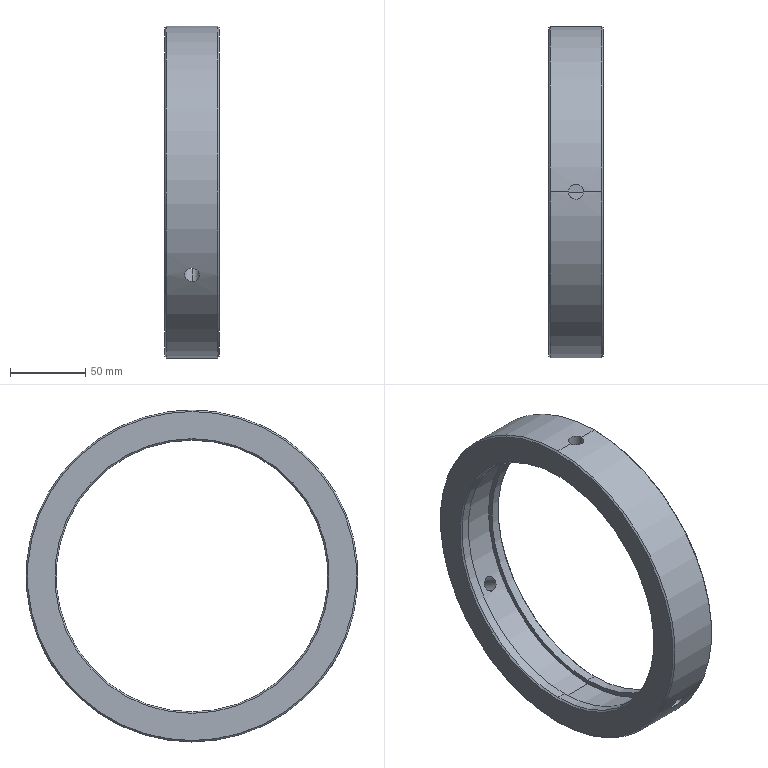Part | SolidWorks | features 3DProfileFeature 1, Chamfer 1, CirPattern 1, HoleWzd 1, Revolution 1 | 1 solid | 26 faces | box 36 x 220 x 220 mm | volume 409173 mm3 | cylinder 14 | cone 8 | plane 4 | commonest cylinder face diameters 10 x6 180 x4 186 x2 220 x2
STEP:
#1=CARTESIAN_POINT('',(0.,-82.924,-42.103));
#2=VERTEX_POINT('',#1);
#3=CARTESIAN_POINT('',(0.,-77.924,-50.763));
#4=VERTEX_POINT('',#3);
#5=CARTESIAN_POINT('',(0.,-82.924,-42.103));
#6=CARTESIAN_POINT('',(-0.3263,-82.924,-42.103));
#7=CARTESIAN_POINT('',(-0.6506,-82.91,-42.131));
#8=CARTESIAN_POINT('',(-1.295,-82.851,-42.245));
#9=CARTESIAN_POINT('',(-1.611,-82.808,-42.331));
#10=CARTESIAN_POINT('',(-2.213,-82.694,-42.553));
#11=CARTESIAN_POINT('',(-2.503,-82.623,-42.69));
#12=CARTESIAN_POINT('',(-3.051,-82.455,-43.015));
#13=CARTESIAN_POINT('',(-3.302,-82.359,-43.198));
#14=CARTESIAN_POINT('',(-3.764,-82.144,-43.606));
#15=CARTESIAN_POINT('',(-3.975,-82.023,-43.833));
#16=CARTESIAN_POINT('',(-4.338,-81.765,-44.312));
#17=CARTESIAN_POINT('',(-4.492,-81.628,-44.564));
#18=CARTESIAN_POINT('',(-4.743,-81.336,-45.094));
#19=CARTESIAN_POINT('',(-4.84,-81.182,-45.372));
#20=CARTESIAN_POINT('',(-4.967,-80.868,-45.929));
#21=CARTESIAN_POINT('',(-5.,-80.707,-46.211));
#22=CARTESIAN_POINT('',(-5.,-80.378,-46.782));
#23=CARTESIAN_POINT('',(-4.968,-80.213,-47.064));
#24=CARTESIAN_POINT('',(-4.873,-79.969,-47.476));
#25=CARTESIAN_POINT('',(-4.834,-79.888,-47.612));
#26=CARTESIAN_POINT('',(-4.739,-79.727,-47.882));
#27=CARTESIAN_POINT('',(-4.683,-79.646,-48.015));
#28=CARTESIAN_POINT('',(-4.495,-79.411,-48.405));
#29=CARTESIAN_POINT('',(-4.342,-79.261,-48.65));
#30=CARTESIAN_POINT('',(-3.98,-78.975,-49.112));
#31=CARTESIAN_POINT('',(-3.769,-78.839,-49.331));
#32=CARTESIAN_POINT('',(-3.307,-78.593,-49.722));
#33=CARTESIAN_POINT('',(-3.056,-78.482,-49.897));
#34=CARTESIAN_POINT('',(-2.511,-78.285,-50.205));
#35=CARTESIAN_POINT('',(-2.219,-78.2,-50.336));
#36=CARTESIAN_POINT('',(-1.618,-78.065,-50.546));
#37=CARTESIAN_POINT('',(-1.304,-78.012,-50.627));
#38=CARTESIAN_POINT('',(-0.6572,-77.942,-50.736));
#39=CARTESIAN_POINT('',(-0.3304,-77.924,-50.763));
#40=CARTESIAN_POINT('',(0.,-77.924,-50.763));
#41=B_SPLINE_CURVE_WITH_KNOTS('',3,(#5,#6,#7,#8,#9,#10,#11,#12,#13,#14,#15,#16,#17,#18,#19,#20,#21,#22,#23,#24,#25,#26,#27,#28,#29,#30,#31,#32,#33,#34,#35,#36,#37,#38,#39,#40),.UNSPECIFIED.,.F.,.F.,(4,2,2,2,2,2,2,2,2,2,2,2,2,2,2,2,2,4),(0.01564,0.01661,0.01759,0.01857,0.01954,0.02052,0.0215,0.02247,0.02345,0.02443,0.02492,0.0254,0.02638,0.02736,0.02834,0.02931,0.03029,0.03127),.UNSPECIFIED.);
#42=EDGE_CURVE('',#2,#4,#41,.T.);
#43=ORIENTED_EDGE('',*,*,#42,.F.);
#44=CARTESIAN_POINT('',(0.,-97.664,-50.613));
#45=VERTEX_POINT('',#44);
#46=CARTESIAN_POINT('',(0.,-97.763,-50.67));
#47=DIRECTION('',(0.,-0.866,-0.5));
#48=VECTOR('',#47,1000.);
#49=LINE('',#46,#48);
#50=EDGE_CURVE('',#2,#45,#49,.T.);
#51=ORIENTED_EDGE('',*,*,#50,.T.);
#52=CARTESIAN_POINT('',(0.,-92.664,-59.273));
#53=VERTEX_POINT('',#52);
#54=CARTESIAN_POINT('',(0.,-92.664,-59.273));
#55=CARTESIAN_POINT('',(-0.3304,-92.664,-59.273));
#56=CARTESIAN_POINT('',(-0.6553,-92.682,-59.246));
#57=CARTESIAN_POINT('',(-1.135,-92.733,-59.166));
#58=CARTESIAN_POINT('',(-1.293,-92.754,-59.132));
#59=CARTESIAN_POINT('',(-1.607,-92.806,-59.052));
#60=CARTESIAN_POINT('',(-1.763,-92.836,-59.005));
#61=CARTESIAN_POINT('',(-2.218,-92.937,-58.845));
#62=CARTESIAN_POINT('',(-2.505,-93.019,-58.716));
#63=CARTESIAN_POINT('',(-3.048,-93.212,-58.408));
#64=CARTESIAN_POINT('',(-3.306,-93.324,-58.229));
#65=CARTESIAN_POINT('',(-3.767,-93.568,-57.837));
#66=CARTESIAN_POINT('',(-3.974,-93.7,-57.623));
#67=CARTESIAN_POINT('',(-4.339,-93.985,-57.156));
#68=CARTESIAN_POINT('',(-4.495,-94.136,-56.907));
#69=CARTESIAN_POINT('',(-4.744,-94.446,-56.391));
#70=CARTESIAN_POINT('',(-4.84,-94.608,-56.12));
#71=CARTESIAN_POINT('',(-4.968,-94.935,-55.564));
#72=CARTESIAN_POINT('',(-5.,-95.099,-55.284));
#73=CARTESIAN_POINT('',(-5.,-95.425,-54.719));
#74=CARTESIAN_POINT('',(-4.968,-95.589,-54.431));
#75=CARTESIAN_POINT('',(-4.84,-95.905,-53.873));
#76=CARTESIAN_POINT('',(-4.745,-96.057,-53.601));
#77=CARTESIAN_POINT('',(-4.495,-96.351,-53.072));
#78=CARTESIAN_POINT('',(-4.338,-96.492,-52.815));
#79=CARTESIAN_POINT('',(-3.976,-96.751,-52.339));
#80=CARTESIAN_POINT('',(-3.77,-96.871,-52.116));
#81=CARTESIAN_POINT('',(-3.303,-97.091,-51.705));
#82=CARTESIAN_POINT('',(-3.05,-97.188,-51.521));
#83=CARTESIAN_POINT('',(-2.644,-97.315,-51.281));
#84=CARTESIAN_POINT('',(-2.504,-97.354,-51.207));
#85=CARTESIAN_POINT('',(-2.215,-97.426,-51.069));
#86=CARTESIAN_POINT('',(-2.065,-97.459,-51.007));
#87=CARTESIAN_POINT('',(-1.61,-97.547,-50.84));
#88=CARTESIAN_POINT('',(-1.299,-97.59,-50.756));
#89=CARTESIAN_POINT('',(-0.6578,-97.649,-50.642));
#90=CARTESIAN_POINT('',(-0.3263,-97.664,-50.613));
#91=CARTESIAN_POINT('',(0.,-97.664,-50.613));
#92=B_SPLINE_CURVE_WITH_KNOTS('',3,(#54,#55,#56,#57,#58,#59,#60,#61,#62,#63,#64,#65,#66,#67,#68,#69,#70,#71,#72,#73,#74,#75,#76,#77,#78,#79,#80,#81,#82,#83,#84,#85,#86,#87,#88,#89,#90,#91),.UNSPECIFIED.,.F.,.F.,(4,2,2,2,2,2,2,2,2,2,2,2,2,2,2,2,2,2,4),(0.,0.0009771,0.001466,0.001954,0.002931,0.003909,0.004886,0.005863,0.00684,0.007817,0.008794,0.009771,0.01075,0.01173,0.0127,0.01319,0.01368,0.01466,0.01563),.UNSPECIFIED.);
#93=EDGE_CURVE('',#53,#45,#92,.T.);
#94=ORIENTED_EDGE('',*,*,#93,.F.);
#95=CARTESIAN_POINT('',(0.,-92.763,-59.33));
#96=DIRECTION('',(0.,-0.866,-0.5));
#97=VECTOR('',#96,1000.);
#98=LINE('',#95,#97);
#99=EDGE_CURVE('',#4,#53,#98,.T.);
#100=ORIENTED_EDGE('',*,*,#99,.F.);
#101=EDGE_LOOP('',(#43,#51,#94,#100));
#102=FACE_OUTER_BOUND('',#101,.T.);
#103=CARTESIAN_POINT('',(0.,-95.263,-55.));
#104=DIRECTION('',(0.,-0.866,-0.5));
#105=DIRECTION('',(0.,0.5,-0.866));
#106=AXIS2_PLACEMENT_3D('',#103,#104,#105);
#107=CYLINDRICAL_SURFACE('',#106,5.);
#108=ADVANCED_FACE('',(#102),#107,.F.);
#109=CARTESIAN_POINT('',(0.,77.924,-50.763));
#110=VERTEX_POINT('',#109);
#111=CARTESIAN_POINT('',(0.,82.924,-42.103));
#112=VERTEX_POINT('',#111);
#113=CARTESIAN_POINT('',(0.,77.924,-50.763));
#114=CARTESIAN_POINT('',(-0.3263,77.924,-50.763));
#115=CARTESIAN_POINT('',(-0.6506,77.941,-50.736));
#116=CARTESIAN_POINT('',(-1.295,78.011,-50.629));
#117=CARTESIAN_POINT('',(-1.611,78.063,-50.548));
#118=CARTESIAN_POINT('',(-2.213,78.199,-50.339));
#119=CARTESIAN_POINT('',(-2.503,78.282,-50.209));
#120=CARTESIAN_POINT('',(-3.051,78.479,-49.9));
#121=CARTESIAN_POINT('',(-3.302,78.59,-49.725));
#122=CARTESIAN_POINT('',(-3.764,78.836,-49.335));
#123=CARTESIAN_POINT('',(-3.975,78.972,-49.117));
#124=CARTESIAN_POINT('',(-4.338,79.258,-48.655));
#125=CARTESIAN_POINT('',(-4.492,79.408,-48.41));
#126=CARTESIAN_POINT('',(-4.743,79.721,-47.892));
#127=CARTESIAN_POINT('',(-4.84,79.884,-47.62));
#128=CARTESIAN_POINT('',(-4.967,80.21,-47.069));
#129=CARTESIAN_POINT('',(-5.,80.373,-46.789));
#130=CARTESIAN_POINT('',(-5.,80.703,-46.218));
#131=CARTESIAN_POINT('',(-4.968,80.865,-45.935));
#132=CARTESIAN_POINT('',(-4.873,81.1,-45.517));
#133=CARTESIAN_POINT('',(-4.834,81.177,-45.379));
#134=CARTESIAN_POINT('',(-4.739,81.33,-45.105));
#135=CARTESIAN_POINT('',(-4.683,81.406,-44.968));
#136=CARTESIAN_POINT('',(-4.495,81.625,-44.57));
#137=CARTESIAN_POINT('',(-4.342,81.762,-44.317));
#138=CARTESIAN_POINT('',(-3.98,82.02,-43.839));
#139=CARTESIAN_POINT('',(-3.769,82.141,-43.611));
#140=CARTESIAN_POINT('',(-3.307,82.357,-43.202));
#141=CARTESIAN_POINT('',(-3.056,82.453,-43.019));
#142=CARTESIAN_POINT('',(-2.511,82.621,-42.694));
#143=CARTESIAN_POINT('',(-2.219,82.693,-42.555));
#144=CARTESIAN_POINT('',(-1.618,82.807,-42.333));
#145=CARTESIAN_POINT('',(-1.304,82.85,-42.247));
#146=CARTESIAN_POINT('',(-0.6572,82.909,-42.132));
#147=CARTESIAN_POINT('',(-0.3304,82.924,-42.103));
#148=CARTESIAN_POINT('',(0.,82.924,-42.103));
#149=B_SPLINE_CURVE_WITH_KNOTS('',3,(#113,#114,#115,#116,#117,#118,#119,#120,#121,#122,#123,#124,#125,#126,#127,#128,#129,#130,#131,#132,#133,#134,#135,#136,#137,#138,#139,#140,#141,#142,#143,#144,#145,#146,#147,#148),.UNSPECIFIED.,.F.,.F.,(4,2,2,2,2,2,2,2,2,2,2,2,2,2,2,2,2,4),(0.01564,0.01661,0.01759,0.01857,0.01954,0.02052,0.0215,0.02247,0.02345,0.02443,0.02492,0.0254,0.02638,0.02736,0.02834,0.02931,0.03029,0.03127),.UNSPECIFIED.);
#150=EDGE_CURVE('',#110,#112,#149,.T.);
#151=ORIENTED_EDGE('',*,*,#150,.F.);
#152=CARTESIAN_POINT('',(0.,92.664,-59.273));
#153=VERTEX_POINT('',#152);
#154=CARTESIAN_POINT('',(0.,92.763,-59.33));
#155=DIRECTION('',(0.,0.866,-0.5));
#156=VECTOR('',#155,1000.);
#157=LINE('',#154,#156);
#158=EDGE_CURVE('',#110,#153,#157,.T.);
#159=ORIENTED_EDGE('',*,*,#158,.T.);
#160=CARTESIAN_POINT('',(0.,97.664,-50.613));
#161=VERTEX_POINT('',#160);
#162=CARTESIAN_POINT('',(0.,97.664,-50.613));
#163=CARTESIAN_POINT('',(-0.3304,97.664,-50.613));
#164=CARTESIAN_POINT('',(-0.6553,97.649,-50.642));
#165=CARTESIAN_POINT('',(-1.135,97.605,-50.727));
#166=CARTESIAN_POINT('',(-1.293,97.587,-50.762));
#167=CARTESIAN_POINT('',(-1.607,97.543,-50.846));
#168=CARTESIAN_POINT('',(-1.763,97.517,-50.896));
#169=CARTESIAN_POINT('',(-2.218,97.43,-51.063));
#170=CARTESIAN_POINT('',(-2.505,97.359,-51.199));
#171=CARTESIAN_POINT('',(-3.048,97.189,-51.52));
#172=CARTESIAN_POINT('',(-3.306,97.09,-51.707));
#173=CARTESIAN_POINT('',(-3.767,96.872,-52.114));
#174=CARTESIAN_POINT('',(-3.974,96.753,-52.335));
#175=CARTESIAN_POINT('',(-4.339,96.491,-52.816));
#176=CARTESIAN_POINT('',(-4.495,96.351,-53.071));
#177=CARTESIAN_POINT('',(-4.744,96.059,-53.597));
#178=CARTESIAN_POINT('',(-4.84,95.906,-53.872));
#179=CARTESIAN_POINT('',(-4.968,95.588,-54.434));
#180=CARTESIAN_POINT('',(-5.,95.427,-54.716));
#181=CARTESIAN_POINT('',(-5.,95.101,-55.281));
#182=CARTESIAN_POINT('',(-4.968,94.934,-55.567));
#183=CARTESIAN_POINT('',(-4.84,94.608,-56.12));
#184=CARTESIAN_POINT('',(-4.745,94.449,-56.388));
#185=CARTESIAN_POINT('',(-4.495,94.137,-56.907));
#186=CARTESIAN_POINT('',(-4.338,93.985,-57.157));
#187=CARTESIAN_POINT('',(-3.976,93.702,-57.619));
#188=CARTESIAN_POINT('',(-3.77,93.569,-57.834));
#189=CARTESIAN_POINT('',(-3.303,93.323,-58.231));
#190=CARTESIAN_POINT('',(-3.05,93.213,-58.407));
#191=CARTESIAN_POINT('',(-2.644,93.068,-58.637));
#192=CARTESIAN_POINT('',(-2.504,93.023,-58.708));
#193=CARTESIAN_POINT('',(-2.215,92.941,-58.839));
#194=CARTESIAN_POINT('',(-2.065,92.903,-58.899));
#195=CARTESIAN_POINT('',(-1.61,92.802,-59.058));
#196=CARTESIAN_POINT('',(-1.299,92.751,-59.138));
#197=CARTESIAN_POINT('',(-0.6578,92.682,-59.246));
#198=CARTESIAN_POINT('',(-0.3263,92.664,-59.273));
#199=CARTESIAN_POINT('',(0.,92.664,-59.273));
#200=B_SPLINE_CURVE_WITH_KNOTS('',3,(#162,#163,#164,#165,#166,#167,#168,#169,#170,#171,#172,#173,#174,#175,#176,#177,#178,#179,#180,#181,#182,#183,#184,#185,#186,#187,#188,#189,#190,#191,#192,#193,#194,#195,#196,#197,#198,#199),.UNSPECIFIED.,.F.,.F.,(4,2,2,2,2,2,2,2,2,2,2,2,2,2,2,2,2,2,4),(0.,0.0009771,0.001466,0.001954,0.002931,0.003909,0.004886,0.005863,0.00684,0.007817,0.008794,0.009771,0.01075,0.01173,0.0127,0.01319,0.01368,0.01466,0.01563),.UNSPECIFIED.);
#201=EDGE_CURVE('',#161,#153,#200,.T.);
#202=ORIENTED_EDGE('',*,*,#201,.F.);
#203=CARTESIAN_POINT('',(0.,97.763,-50.67));
#204=DIRECTION('',(0.,0.866,-0.5));
#205=VECTOR('',#204,1000.);
#206=LINE('',#203,#205);
#207=EDGE_CURVE('',#112,#161,#206,.T.);
#208=ORIENTED_EDGE('',*,*,#207,.F.);
#209=EDGE_LOOP('',(#151,#159,#202,#208));
#210=FACE_OUTER_BOUND('',#209,.T.);
#211=CARTESIAN_POINT('',(0.,95.263,-55.));
#212=DIRECTION('',(0.,0.866,-0.5));
#213=DIRECTION('',(0.,0.5,0.866));
#214=AXIS2_PLACEMENT_3D('',#211,#212,#213);
#215=CYLINDRICAL_SURFACE('',#214,5.);
#216=ADVANCED_FACE('',(#210),#215,.F.);
#217=CARTESIAN_POINT('',(-5.,0.,93.));
#218=VERTEX_POINT('',#217);
#219=CARTESIAN_POINT('',(5.,0.,93.));
#220=VERTEX_POINT('',#219);
#221=CARTESIAN_POINT('',(-5.,0.,93.));
#222=CARTESIAN_POINT('',(-5.,-0.3263,93.));
#223=CARTESIAN_POINT('',(-4.968,-0.6506,92.998));
#224=CARTESIAN_POINT('',(-4.84,-1.295,92.992));
#225=CARTESIAN_POINT('',(-4.744,-1.611,92.987));
#226=CARTESIAN_POINT('',(-4.495,-2.213,92.974));
#227=CARTESIAN_POINT('',(-4.341,-2.503,92.967));
#228=CARTESIAN_POINT('',(-3.975,-3.051,92.95));
#229=CARTESIAN_POINT('',(-3.768,-3.302,92.942));
#230=CARTESIAN_POINT('',(-3.308,-3.764,92.924));
#231=CARTESIAN_POINT('',(-3.051,-3.975,92.915));
#232=CARTESIAN_POINT('',(-2.507,-4.338,92.899));
#233=CARTESIAN_POINT('',(-2.22,-4.492,92.892));
#234=CARTESIAN_POINT('',(-1.616,-4.743,92.879));
#235=CARTESIAN_POINT('',(-1.298,-4.84,92.874));
#236=CARTESIAN_POINT('',(-0.6586,-4.967,92.867));
#237=CARTESIAN_POINT('',(-0.3339,-5.,92.866));
#238=CARTESIAN_POINT('',(0.3257,-5.,92.865));
#239=CARTESIAN_POINT('',(0.6518,-4.968,92.867));
#240=CARTESIAN_POINT('',(1.131,-4.873,92.872));
#241=CARTESIAN_POINT('',(1.289,-4.834,92.874));
#242=CARTESIAN_POINT('',(1.603,-4.739,92.879));
#243=CARTESIAN_POINT('',(1.759,-4.683,92.882));
#244=CARTESIAN_POINT('',(2.214,-4.495,92.891));
#245=CARTESIAN_POINT('',(2.501,-4.342,92.899));
#246=CARTESIAN_POINT('',(3.045,-3.98,92.915));
#247=CARTESIAN_POINT('',(3.302,-3.769,92.924));
#248=CARTESIAN_POINT('',(3.764,-3.307,92.941));
#249=CARTESIAN_POINT('',(3.971,-3.056,92.95));
#250=CARTESIAN_POINT('',(4.336,-2.511,92.967));
#251=CARTESIAN_POINT('',(4.492,-2.219,92.974));
#252=CARTESIAN_POINT('',(4.742,-1.618,92.986));
#253=CARTESIAN_POINT('',(4.838,-1.304,92.991));
#254=CARTESIAN_POINT('',(4.968,-0.6572,92.998));
#255=CARTESIAN_POINT('',(5.,-0.3304,93.));
#256=CARTESIAN_POINT('',(5.,0.,93.));
#257=B_SPLINE_CURVE_WITH_KNOTS('',3,(#221,#222,#223,#224,#225,#226,#227,#228,#229,#230,#231,#232,#233,#234,#235,#236,#237,#238,#239,#240,#241,#242,#243,#244,#245,#246,#247,#248,#249,#250,#251,#252,#253,#254,#255,#256),.UNSPECIFIED.,.F.,.F.,(4,2,2,2,2,2,2,2,2,2,2,2,2,2,2,2,2,4),(0.01564,0.01661,0.01759,0.01857,0.01954,0.02052,0.0215,0.02247,0.02345,0.02443,0.02492,0.0254,0.02638,0.02736,0.02834,0.02931,0.03029,0.03127),.UNSPECIFIED.);
#258=EDGE_CURVE('',#218,#220,#257,.T.);
#259=ORIENTED_EDGE('',*,*,#258,.F.);
#260=CARTESIAN_POINT('',(-5.,0.,110.));
#261=VERTEX_POINT('',#260);
#262=CARTESIAN_POINT('',(-5.,0.,110.));
#263=DIRECTION('',(0.,0.,1.));
#264=VECTOR('',#263,1000.);
#265=LINE('',#262,#264);
#266=EDGE_CURVE('',#218,#261,#265,.T.);
#267=ORIENTED_EDGE('',*,*,#266,.T.);
#268=CARTESIAN_POINT('',(5.,0.,110.));
#269=VERTEX_POINT('',#268);
#270=CARTESIAN_POINT('',(5.,0.,110.));
#271=CARTESIAN_POINT('',(5.,-0.3304,110.));
#272=CARTESIAN_POINT('',(4.968,-0.6553,109.999));
#273=CARTESIAN_POINT('',(4.872,-1.135,109.994));
#274=CARTESIAN_POINT('',(4.833,-1.293,109.993));
#275=CARTESIAN_POINT('',(4.737,-1.607,109.988));
#276=CARTESIAN_POINT('',(4.682,-1.763,109.986));
#277=CARTESIAN_POINT('',(4.493,-2.218,109.978));
#278=CARTESIAN_POINT('',(4.34,-2.505,109.972));
#279=CARTESIAN_POINT('',(3.977,-3.048,109.958));
#280=CARTESIAN_POINT('',(3.766,-3.306,109.951));
#281=CARTESIAN_POINT('',(3.304,-3.767,109.936));
#282=CARTESIAN_POINT('',(3.052,-3.974,109.928));
#283=CARTESIAN_POINT('',(2.506,-4.339,109.915));
#284=CARTESIAN_POINT('',(2.215,-4.495,109.908));
#285=CARTESIAN_POINT('',(1.613,-4.744,109.898));
#286=CARTESIAN_POINT('',(1.298,-4.84,109.893));
#287=CARTESIAN_POINT('',(0.6524,-4.968,109.888));
#288=CARTESIAN_POINT('',(0.3279,-5.,109.886));
#289=CARTESIAN_POINT('',(-0.3244,-5.,109.886));
#290=CARTESIAN_POINT('',(-0.6557,-4.968,109.888));
#291=CARTESIAN_POINT('',(-1.297,-4.84,109.893));
#292=CARTESIAN_POINT('',(-1.609,-4.745,109.898));
#293=CARTESIAN_POINT('',(-2.214,-4.495,109.908));
#294=CARTESIAN_POINT('',(-2.507,-4.338,109.915));
#295=CARTESIAN_POINT('',(-3.049,-3.976,109.928));
#296=CARTESIAN_POINT('',(-3.301,-3.77,109.936));
#297=CARTESIAN_POINT('',(-3.768,-3.303,109.951));
#298=CARTESIAN_POINT('',(-3.975,-3.05,109.958));
#299=CARTESIAN_POINT('',(-4.247,-2.644,109.968));
#300=CARTESIAN_POINT('',(-4.331,-2.504,109.972));
#301=CARTESIAN_POINT('',(-4.486,-2.215,109.978));
#302=CARTESIAN_POINT('',(-4.557,-2.065,109.981));
#303=CARTESIAN_POINT('',(-4.745,-1.61,109.989));
#304=CARTESIAN_POINT('',(-4.839,-1.299,109.993));
#305=CARTESIAN_POINT('',(-4.967,-0.6578,109.998));
#306=CARTESIAN_POINT('',(-5.,-0.3263,110.));
#307=CARTESIAN_POINT('',(-5.,0.,110.));
#308=B_SPLINE_CURVE_WITH_KNOTS('',3,(#270,#271,#272,#273,#274,#275,#276,#277,#278,#279,#280,#281,#282,#283,#284,#285,#286,#287,#288,#289,#290,#291,#292,#293,#294,#295,#296,#297,#298,#299,#300,#301,#302,#303,#304,#305,#306,#307),.UNSPECIFIED.,.F.,.F.,(4,2,2,2,2,2,2,2,2,2,2,2,2,2,2,2,2,2,4),(0.,0.0009771,0.001466,0.001954,0.002931,0.003909,0.004886,0.005863,0.00684,0.007817,0.008794,0.009771,0.01075,0.01173,0.0127,0.01319,0.01368,0.01466,0.01563),.UNSPECIFIED.);
#309=EDGE_CURVE('',#269,#261,#308,.T.);
#310=ORIENTED_EDGE('',*,*,#309,.F.);
#311=CARTESIAN_POINT('',(5.,0.,110.));
#312=DIRECTION('',(0.,0.,1.));
#313=VECTOR('',#312,1000.);
#314=LINE('',#311,#313);
#315=EDGE_CURVE('',#220,#269,#314,.T.);
#316=ORIENTED_EDGE('',*,*,#315,.F.);
#317=EDGE_LOOP('',(#259,#267,#310,#316));
#318=FACE_OUTER_BOUND('',#317,.T.);
#319=CARTESIAN_POINT('',(0.,0.,110.));
#320=DIRECTION('',(0.,0.,1.));
#321=DIRECTION('',(1.,0.,0.));
#322=AXIS2_PLACEMENT_3D('',#319,#320,#321);
#323=CYLINDRICAL_SURFACE('',#322,5.);
#324=ADVANCED_FACE('',(#318),#323,.F.);
#325=CARTESIAN_POINT('',(18.,0.,-109.));
#326=VERTEX_POINT('',#325);
#327=CARTESIAN_POINT('',(18.,0.,109.));
#328=VERTEX_POINT('',#327);
#329=CARTESIAN_POINT('',(18.,0.,0.));
#330=DIRECTION('',(1.,0.,0.));
#331=DIRECTION('',(0.,0.,1.));
#332=AXIS2_PLACEMENT_3D('',#329,#330,#331);
#333=CIRCLE('',#332,109.);
#334=EDGE_CURVE('',#326,#328,#333,.T.);
#335=ORIENTED_EDGE('',*,*,#334,.F.);
#336=CARTESIAN_POINT('',(17.,0.,-110.));
#337=VERTEX_POINT('',#336);
#338=CARTESIAN_POINT('',(17.,0.,-110.));
#339=DIRECTION('',(-0.7071,0.,-0.7071));
#340=VECTOR('',#339,1000.);
#341=LINE('',#338,#340);
#342=EDGE_CURVE('',#326,#337,#341,.T.);
#343=ORIENTED_EDGE('',*,*,#342,.T.);
#344=CARTESIAN_POINT('',(17.,0.,110.));
#345=VERTEX_POINT('',#344);
#346=CARTESIAN_POINT('',(17.,0.,0.));
#347=DIRECTION('',(-1.,0.,0.));
#348=DIRECTION('',(0.,0.,1.));
#349=AXIS2_PLACEMENT_3D('',#346,#347,#348);
#350=CIRCLE('',#349,110.);
#351=EDGE_CURVE('',#345,#337,#350,.T.);
#352=ORIENTED_EDGE('',*,*,#351,.F.);
#353=CARTESIAN_POINT('',(17.,0.,110.));
#354=DIRECTION('',(-0.7071,0.,0.7071));
#355=VECTOR('',#354,1000.);
#356=LINE('',#353,#355);
#357=EDGE_CURVE('',#328,#345,#356,.T.);
#358=ORIENTED_EDGE('',*,*,#357,.F.);
#359=EDGE_LOOP('',(#335,#343,#352,#358));
#360=FACE_OUTER_BOUND('',#359,.T.);
#361=CARTESIAN_POINT('',(17.,0.,0.));
#362=DIRECTION('',(-1.,0.,0.));
#363=DIRECTION('',(0.,0.,1.));
#364=AXIS2_PLACEMENT_3D('',#361,#362,#363);
#365=CONICAL_SURFACE('',#364,110.,0.7854);
#366=ADVANCED_FACE('',(#360),#365,.T.);
#367=CARTESIAN_POINT('',(17.,0.,90.));
#368=VERTEX_POINT('',#367);
#369=CARTESIAN_POINT('',(17.,0.,-90.));
#370=VERTEX_POINT('',#369);
#371=CARTESIAN_POINT('',(17.,0.,0.));
#372=DIRECTION('',(1.,0.,0.));
#373=DIRECTION('',(0.,0.,1.));
#374=AXIS2_PLACEMENT_3D('',#371,#372,#373);
#375=CIRCLE('',#374,90.);
#376=EDGE_CURVE('',#368,#370,#375,.T.);
#377=ORIENTED_EDGE('',*,*,#376,.F.);
#378=CARTESIAN_POINT('',(18.,0.,91.));
#379=VERTEX_POINT('',#378);
#380=CARTESIAN_POINT('',(18.,0.,91.));
#381=DIRECTION('',(0.7071,0.,0.7071));
#382=VECTOR('',#381,1000.);
#383=LINE('',#380,#382);
#384=EDGE_CURVE('',#368,#379,#383,.T.);
#385=ORIENTED_EDGE('',*,*,#384,.T.);
#386=CARTESIAN_POINT('',(18.,0.,-91.));
#387=VERTEX_POINT('',#386);
#388=CARTESIAN_POINT('',(18.,0.,0.));
#389=DIRECTION('',(-1.,0.,0.));
#390=DIRECTION('',(0.,0.,1.));
#391=AXIS2_PLACEMENT_3D('',#388,#389,#390);
#392=CIRCLE('',#391,91.);
#393=EDGE_CURVE('',#387,#379,#392,.T.);
#394=ORIENTED_EDGE('',*,*,#393,.F.);
#395=CARTESIAN_POINT('',(18.,0.,-91.));
#396=DIRECTION('',(0.7071,0.,-0.7071));
#397=VECTOR('',#396,1000.);
#398=LINE('',#395,#397);
#399=EDGE_CURVE('',#370,#387,#398,.T.);
#400=ORIENTED_EDGE('',*,*,#399,.F.);
#401=EDGE_LOOP('',(#377,#385,#394,#400));
#402=FACE_OUTER_BOUND('',#401,.T.);
#403=CARTESIAN_POINT('',(18.,0.,0.));
#404=DIRECTION('',(1.,0.,0.));
#405=DIRECTION('',(0.,0.,-1.));
#406=AXIS2_PLACEMENT_3D('',#403,#404,#405);
#407=CONICAL_SURFACE('',#406,91.,0.7854);
#408=ADVANCED_FACE('',(#402),#407,.F.);
#409=CARTESIAN_POINT('',(-17.,0.,-90.));
#410=VERTEX_POINT('',#409);
#411=CARTESIAN_POINT('',(-17.,0.,90.));
#412=VERTEX_POINT('',#411);
#413=CARTESIAN_POINT('',(-17.,0.,0.));
#414=DIRECTION('',(-1.,0.,0.));
#415=DIRECTION('',(0.,0.,-1.));
#416=AXIS2_PLACEMENT_3D('',#413,#414,#415);
#417=CIRCLE('',#416,90.);
#418=EDGE_CURVE('',#410,#412,#417,.T.);
#419=ORIENTED_EDGE('',*,*,#418,.F.);
#420=CARTESIAN_POINT('',(-18.,0.,-91.));
#421=VERTEX_POINT('',#420);
#422=CARTESIAN_POINT('',(-17.,0.,-90.));
#423=DIRECTION('',(-0.7071,0.,-0.7071));
#424=VECTOR('',#423,1000.);
#425=LINE('',#422,#424);
#426=EDGE_CURVE('',#410,#421,#425,.T.);
#427=ORIENTED_EDGE('',*,*,#426,.T.);
#428=CARTESIAN_POINT('',(-18.,0.,91.));
#429=VERTEX_POINT('',#428);
#430=CARTESIAN_POINT('',(-18.,0.,0.));
#431=DIRECTION('',(1.,0.,0.));
#432=DIRECTION('',(0.,0.,-1.));
#433=AXIS2_PLACEMENT_3D('',#430,#431,#432);
#434=CIRCLE('',#433,91.);
#435=EDGE_CURVE('',#429,#421,#434,.T.);
#436=ORIENTED_EDGE('',*,*,#435,.F.);
#437=CARTESIAN_POINT('',(-17.,0.,90.));
#438=DIRECTION('',(-0.7071,0.,0.7071));
#439=VECTOR('',#438,1000.);
#440=LINE('',#437,#439);
#441=EDGE_CURVE('',#412,#429,#440,.T.);
#442=ORIENTED_EDGE('',*,*,#441,.F.);
#443=EDGE_LOOP('',(#419,#427,#436,#442));
#444=FACE_OUTER_BOUND('',#443,.T.);
#445=CARTESIAN_POINT('',(-17.,0.,0.));
#446=DIRECTION('',(-1.,0.,0.));
#447=DIRECTION('',(0.,0.,1.));
#448=AXIS2_PLACEMENT_3D('',#445,#446,#447);
#449=CONICAL_SURFACE('',#448,90.,0.7854);
#450=ADVANCED_FACE('',(#444),#449,.F.);
#451=CARTESIAN_POINT('',(-18.,0.,109.));
#452=VERTEX_POINT('',#451);
#453=CARTESIAN_POINT('',(-18.,0.,-109.));
#454=VERTEX_POINT('',#453);
#455=CARTESIAN_POINT('',(-18.,0.,0.));
#456=DIRECTION('',(-1.,0.,0.));
#457=DIRECTION('',(0.,0.,-1.));
#458=AXIS2_PLACEMENT_3D('',#455,#456,#457);
#459=CIRCLE('',#458,109.);
#460=EDGE_CURVE('',#452,#454,#459,.T.);
#461=ORIENTED_EDGE('',*,*,#460,.F.);
#462=CARTESIAN_POINT('',(-17.,0.,110.));
#463=VERTEX_POINT('',#462);
#464=CARTESIAN_POINT('',(-18.,0.,109.));
#465=DIRECTION('',(0.7071,0.,0.7071));
#466=VECTOR('',#465,1000.);
#467=LINE('',#464,#466);
#468=EDGE_CURVE('',#452,#463,#467,.T.);
#469=ORIENTED_EDGE('',*,*,#468,.T.);
#470=CARTESIAN_POINT('',(-17.,0.,-110.));
#471=VERTEX_POINT('',#470);
#472=CARTESIAN_POINT('',(-17.,0.,0.));
#473=DIRECTION('',(1.,0.,0.));
#474=DIRECTION('',(0.,0.,-1.));
#475=AXIS2_PLACEMENT_3D('',#472,#473,#474);
#476=CIRCLE('',#475,110.);
#477=EDGE_CURVE('',#471,#463,#476,.T.);
#478=ORIENTED_EDGE('',*,*,#477,.F.);
#479=CARTESIAN_POINT('',(-18.,0.,-109.));
#480=DIRECTION('',(0.7071,0.,-0.7071));
#481=VECTOR('',#480,1000.);
#482=LINE('',#479,#481);
#483=EDGE_CURVE('',#454,#471,#482,.T.);
#484=ORIENTED_EDGE('',*,*,#483,.F.);
#485=EDGE_LOOP('',(#461,#469,#478,#484));
#486=FACE_OUTER_BOUND('',#485,.T.);
#487=CARTESIAN_POINT('',(-18.,0.,0.));
#488=DIRECTION('',(1.,0.,0.));
#489=DIRECTION('',(0.,0.,-1.));
#490=AXIS2_PLACEMENT_3D('',#487,#488,#489);
#491=CONICAL_SURFACE('',#490,109.,0.7854);
#492=ADVANCED_FACE('',(#486),#491,.T.);
#493=CARTESIAN_POINT('',(-11.,0.,-90.));
#494=VERTEX_POINT('',#493);
#495=CARTESIAN_POINT('',(-11.,0.,90.));
#496=VERTEX_POINT('',#495);
#497=CARTESIAN_POINT('',(-11.,0.,0.));
#498=DIRECTION('',(-1.,0.,0.));
#499=DIRECTION('',(0.,0.,1.));
#500=AXIS2_PLACEMENT_3D('',#497,#498,#499);
#501=CIRCLE('',#500,90.);
#502=EDGE_CURVE('',#494,#496,#501,.T.);
#503=ORIENTED_EDGE('',*,*,#502,.F.);
#504=CARTESIAN_POINT('',(-24.333,0.,-90.));
#505=DIRECTION('',(-1.,0.,0.));
#506=VECTOR('',#505,1000.);
#507=LINE('',#504,#506);
#508=EDGE_CURVE('',#494,#410,#507,.T.);
#509=ORIENTED_EDGE('',*,*,#508,.T.);
#510=ORIENTED_EDGE('',*,*,#418,.T.);
#511=CARTESIAN_POINT('',(-24.333,0.,90.));
#512=DIRECTION('',(-1.,0.,0.));
#513=VECTOR('',#512,1000.);
#514=LINE('',#511,#513);
#515=EDGE_CURVE('',#496,#412,#514,.T.);
#516=ORIENTED_EDGE('',*,*,#515,.F.);
#517=EDGE_LOOP('',(#503,#509,#510,#516));
#518=FACE_OUTER_BOUND('',#517,.T.);
#519=CARTESIAN_POINT('',(-24.333,0.,0.));
#520=DIRECTION('',(-1.,0.,0.));
#521=DIRECTION('',(0.,0.,1.));
#522=AXIS2_PLACEMENT_3D('',#519,#520,#521);
#523=CYLINDRICAL_SURFACE('',#522,90.);
#524=ADVANCED_FACE('',(#518),#523,.F.);
#525=CARTESIAN_POINT('',(0.,-77.924,-50.763));
#526=CARTESIAN_POINT('',(0.3304,-77.924,-50.763));
#527=CARTESIAN_POINT('',(0.6553,-77.942,-50.736));
#528=CARTESIAN_POINT('',(1.135,-77.994,-50.656));
#529=CARTESIAN_POINT('',(1.293,-78.015,-50.622));
#530=CARTESIAN_POINT('',(1.607,-78.067,-50.542));
#531=CARTESIAN_POINT('',(1.763,-78.097,-50.495));
#532=CARTESIAN_POINT('',(2.218,-78.2,-50.337));
#533=CARTESIAN_POINT('',(2.505,-78.283,-50.208));
#534=CARTESIAN_POINT('',(3.048,-78.478,-49.902));
#535=CARTESIAN_POINT('',(3.306,-78.592,-49.723));
#536=CARTESIAN_POINT('',(3.767,-78.838,-49.332));
#537=CARTESIAN_POINT('',(3.974,-78.971,-49.119));
#538=CARTESIAN_POINT('',(4.339,-79.259,-48.653));
#539=CARTESIAN_POINT('',(4.494,-79.411,-48.405));
#540=CARTESIAN_POINT('',(4.744,-79.722,-47.89));
#541=CARTESIAN_POINT('',(4.84,-79.884,-47.62));
#542=CARTESIAN_POINT('',(4.968,-80.213,-47.064));
#543=CARTESIAN_POINT('',(5.,-80.376,-46.784));
#544=CARTESIAN_POINT('',(5.,-80.703,-46.219));
#545=CARTESIAN_POINT('',(4.968,-80.867,-45.931));
#546=CARTESIAN_POINT('',(4.84,-81.182,-45.372));
#547=CARTESIAN_POINT('',(4.745,-81.333,-45.1));
#548=CARTESIAN_POINT('',(4.495,-81.625,-44.569));
#549=CARTESIAN_POINT('',(4.338,-81.765,-44.312));
#550=CARTESIAN_POINT('',(3.976,-82.022,-43.835));
#551=CARTESIAN_POINT('',(3.77,-82.141,-43.612));
#552=CARTESIAN_POINT('',(3.303,-82.359,-43.199));
#553=CARTESIAN_POINT('',(3.05,-82.455,-43.015));
#554=CARTESIAN_POINT('',(2.644,-82.58,-42.774));
#555=CARTESIAN_POINT('',(2.504,-82.618,-42.699));
#556=CARTESIAN_POINT('',(2.215,-82.69,-42.561));
#557=CARTESIAN_POINT('',(2.065,-82.722,-42.498));
#558=CARTESIAN_POINT('',(1.61,-82.808,-42.33));
#559=CARTESIAN_POINT('',(1.299,-82.851,-42.246));
#560=CARTESIAN_POINT('',(0.6578,-82.909,-42.132));
#561=CARTESIAN_POINT('',(0.3264,-82.924,-42.103));
#562=CARTESIAN_POINT('',(0.,-82.924,-42.103));
#563=B_SPLINE_CURVE_WITH_KNOTS('',3,(#525,#526,#527,#528,#529,#530,#531,#532,#533,#534,#535,#536,#537,#538,#539,#540,#541,#542,#543,#544,#545,#546,#547,#548,#549,#550,#551,#552,#553,#554,#555,#556,#557,#558,#559,#560,#561,#562),.UNSPECIFIED.,.F.,.F.,(4,2,2,2,2,2,2,2,2,2,2,2,2,2,2,2,2,2,4),(0.,0.0009772,0.001466,0.001954,0.002932,0.003909,0.004886,0.005863,0.00684,0.007818,0.008795,0.009772,0.01075,0.01173,0.0127,0.01319,0.01368,0.01466,0.01564),.UNSPECIFIED.);
#564=EDGE_CURVE('',#4,#2,#563,.T.);
#565=ORIENTED_EDGE('',*,*,#564,.T.);
#566=ORIENTED_EDGE('',*,*,#42,.T.);
#567=EDGE_LOOP('',(#565,#566));
#568=FACE_BOUND('',#567,.T.);
#569=CARTESIAN_POINT('',(11.,0.,-93.));
#570=VERTEX_POINT('',#569);
#571=CARTESIAN_POINT('',(11.,0.,93.));
#572=VERTEX_POINT('',#571);
#573=CARTESIAN_POINT('',(11.,0.,0.));
#574=DIRECTION('',(-1.,0.,0.));
#575=DIRECTION('',(0.,0.,1.));
#576=AXIS2_PLACEMENT_3D('',#573,#574,#575);
#577=CIRCLE('',#576,93.);
#578=EDGE_CURVE('',#570,#572,#577,.T.);
#579=ORIENTED_EDGE('',*,*,#578,.F.);
#580=CARTESIAN_POINT('',(-11.,0.,-93.));
#581=VERTEX_POINT('',#580);
#582=CARTESIAN_POINT('',(-24.333,0.,-93.));
#583=DIRECTION('',(-1.,0.,0.));
#584=VECTOR('',#583,1000.);
#585=LINE('',#582,#584);
#586=EDGE_CURVE('',#570,#581,#585,.T.);
#587=ORIENTED_EDGE('',*,*,#586,.T.);
#588=CARTESIAN_POINT('',(-11.,0.,93.));
#589=VERTEX_POINT('',#588);
#590=CARTESIAN_POINT('',(-11.,0.,0.));
#591=DIRECTION('',(-1.,0.,0.));
#592=DIRECTION('',(0.,0.,1.));
#593=AXIS2_PLACEMENT_3D('',#590,#591,#592);
#594=CIRCLE('',#593,93.);
#595=EDGE_CURVE('',#581,#589,#594,.T.);
#596=ORIENTED_EDGE('',*,*,#595,.T.);
#597=CARTESIAN_POINT('',(-24.333,0.,93.));
#598=DIRECTION('',(-1.,0.,0.));
#599=VECTOR('',#598,1000.);
#600=LINE('',#597,#599);
#601=EDGE_CURVE('',#218,#589,#600,.T.);
#602=ORIENTED_EDGE('',*,*,#601,.F.);
#603=ORIENTED_EDGE('',*,*,#258,.T.);
#604=CARTESIAN_POINT('',(-24.333,0.,93.));
#605=DIRECTION('',(-1.,0.,0.));
#606=VECTOR('',#605,1000.);
#607=LINE('',#604,#606);
#608=EDGE_CURVE('',#572,#220,#607,.T.);
#609=ORIENTED_EDGE('',*,*,#608,.F.);
#610=EDGE_LOOP('',(#579,#587,#596,#602,#603,#609));
#611=FACE_OUTER_BOUND('',#610,.T.);
#612=CARTESIAN_POINT('',(-24.333,0.,0.));
#613=DIRECTION('',(-1.,0.,0.));
#614=DIRECTION('',(0.,0.,1.));
#615=AXIS2_PLACEMENT_3D('',#612,#613,#614);
#616=CYLINDRICAL_SURFACE('',#615,93.);
#617=ADVANCED_FACE('',(#568,#611),#616,.F.);
#618=ORIENTED_EDGE('',*,*,#376,.T.);
#619=CARTESIAN_POINT('',(11.,0.,-90.));
#620=VERTEX_POINT('',#619);
#621=CARTESIAN_POINT('',(-24.333,0.,-90.));
#622=DIRECTION('',(-1.,0.,0.));
#623=VECTOR('',#622,1000.);
#624=LINE('',#621,#623);
#625=EDGE_CURVE('',#370,#620,#624,.T.);
#626=ORIENTED_EDGE('',*,*,#625,.T.);
#627=CARTESIAN_POINT('',(11.,0.,90.));
#628=VERTEX_POINT('',#627);
#629=CARTESIAN_POINT('',(11.,0.,0.));
#630=DIRECTION('',(-1.,0.,0.));
#631=DIRECTION('',(0.,0.,1.));
#632=AXIS2_PLACEMENT_3D('',#629,#630,#631);
#633=CIRCLE('',#632,90.);
#634=EDGE_CURVE('',#620,#628,#633,.T.);
#635=ORIENTED_EDGE('',*,*,#634,.T.);
#636=CARTESIAN_POINT('',(-24.333,0.,90.));
#637=DIRECTION('',(-1.,0.,0.));
#638=VECTOR('',#637,1000.);
#639=LINE('',#636,#638);
#640=EDGE_CURVE('',#368,#628,#639,.T.);
#641=ORIENTED_EDGE('',*,*,#640,.F.);
#642=EDGE_LOOP('',(#618,#626,#635,#641));
#643=FACE_OUTER_BOUND('',#642,.T.);
#644=CARTESIAN_POINT('',(-24.333,0.,0.));
#645=DIRECTION('',(-1.,0.,0.));
#646=DIRECTION('',(0.,0.,1.));
#647=AXIS2_PLACEMENT_3D('',#644,#645,#646);
#648=CYLINDRICAL_SURFACE('',#647,90.);
#649=ADVANCED_FACE('',(#643),#648,.F.);
#650=ORIENTED_EDGE('',*,*,#201,.T.);
#651=CARTESIAN_POINT('',(0.,92.664,-59.273));
#652=CARTESIAN_POINT('',(0.3263,92.664,-59.273));
#653=CARTESIAN_POINT('',(0.6506,92.681,-59.247));
#654=CARTESIAN_POINT('',(1.295,92.75,-59.139));
#655=CARTESIAN_POINT('',(1.611,92.802,-59.058));
#656=CARTESIAN_POINT('',(2.213,92.936,-58.847));
#657=CARTESIAN_POINT('',(2.503,93.018,-58.717));
#658=CARTESIAN_POINT('',(3.051,93.213,-58.407));
#659=CARTESIAN_POINT('',(3.302,93.323,-58.231));
#660=CARTESIAN_POINT('',(3.764,93.566,-57.84));
#661=CARTESIAN_POINT('',(3.975,93.701,-57.621));
#662=CARTESIAN_POINT('',(4.338,93.985,-57.157));
#663=CARTESIAN_POINT('',(4.492,94.134,-56.912));
#664=CARTESIAN_POINT('',(4.743,94.445,-56.393));
#665=CARTESIAN_POINT('',(4.84,94.608,-56.12));
#666=CARTESIAN_POINT('',(4.967,94.932,-55.57));
#667=CARTESIAN_POINT('',(5.,95.096,-55.289));
#668=CARTESIAN_POINT('',(5.,95.426,-54.718));
#669=CARTESIAN_POINT('',(4.968,95.587,-54.435));
#670=CARTESIAN_POINT('',(4.873,95.823,-54.018));
#671=CARTESIAN_POINT('',(4.834,95.901,-53.88));
#672=CARTESIAN_POINT('',(4.739,96.054,-53.606));
#673=CARTESIAN_POINT('',(4.683,96.13,-53.469));
#674=CARTESIAN_POINT('',(4.495,96.351,-53.072));
#675=CARTESIAN_POINT('',(4.342,96.489,-52.82));
#676=CARTESIAN_POINT('',(3.98,96.749,-52.342));
#677=CARTESIAN_POINT('',(3.769,96.871,-52.116));
#678=CARTESIAN_POINT('',(3.307,97.089,-51.708));
#679=CARTESIAN_POINT('',(3.056,97.186,-51.525));
#680=CARTESIAN_POINT('',(2.511,97.357,-51.202));
#681=CARTESIAN_POINT('',(2.219,97.43,-51.064));
#682=CARTESIAN_POINT('',(1.618,97.545,-50.842));
#683=CARTESIAN_POINT('',(1.304,97.59,-50.757));
#684=CARTESIAN_POINT('',(0.6572,97.649,-50.642));
#685=CARTESIAN_POINT('',(0.3303,97.664,-50.613));
#686=CARTESIAN_POINT('',(0.,97.664,-50.613));
#687=B_SPLINE_CURVE_WITH_KNOTS('',3,(#651,#652,#653,#654,#655,#656,#657,#658,#659,#660,#661,#662,#663,#664,#665,#666,#667,#668,#669,#670,#671,#672,#673,#674,#675,#676,#677,#678,#679,#680,#681,#682,#683,#684,#685,#686),.UNSPECIFIED.,.F.,.F.,(4,2,2,2,2,2,2,2,2,2,2,2,2,2,2,2,2,4),(0.01563,0.01661,0.01759,0.01857,0.01954,0.02052,0.0215,0.02247,0.02345,0.02443,0.02492,0.0254,0.02638,0.02736,0.02833,0.02931,0.03029,0.03127),.UNSPECIFIED.);
#688=EDGE_CURVE('',#153,#161,#687,.T.);
#689=ORIENTED_EDGE('',*,*,#688,.T.);
#690=EDGE_LOOP('',(#650,#689));
#691=FACE_BOUND('',#690,.T.);
#692=ORIENTED_EDGE('',*,*,#351,.T.);
#693=CARTESIAN_POINT('',(-24.333,0.,-110.));
#694=DIRECTION('',(-1.,0.,0.));
#695=VECTOR('',#694,1000.);
#696=LINE('',#693,#695);
#697=EDGE_CURVE('',#337,#471,#696,.T.);
#698=ORIENTED_EDGE('',*,*,#697,.T.);
#699=ORIENTED_EDGE('',*,*,#477,.T.);
#700=CARTESIAN_POINT('',(-24.333,0.,110.));
#701=DIRECTION('',(-1.,0.,0.));
#702=VECTOR('',#701,1000.);
#703=LINE('',#700,#702);
#704=EDGE_CURVE('',#261,#463,#703,.T.);
#705=ORIENTED_EDGE('',*,*,#704,.F.);
#706=CARTESIAN_POINT('',(-5.,0.,110.));
#707=CARTESIAN_POINT('',(-5.,0.3263,110.));
#708=CARTESIAN_POINT('',(-4.968,0.6506,109.999));
#709=CARTESIAN_POINT('',(-4.841,1.295,109.993));
#710=CARTESIAN_POINT('',(-4.745,1.611,109.989));
#711=CARTESIAN_POINT('',(-4.495,2.213,109.978));
#712=CARTESIAN_POINT('',(-4.341,2.503,109.972));
#713=CARTESIAN_POINT('',(-3.975,3.051,109.958));
#714=CARTESIAN_POINT('',(-3.768,3.302,109.951));
#715=CARTESIAN_POINT('',(-3.308,3.764,109.936));
#716=CARTESIAN_POINT('',(-3.051,3.975,109.928));
#717=CARTESIAN_POINT('',(-2.507,4.338,109.915));
#718=CARTESIAN_POINT('',(-2.22,4.492,109.908));
#719=CARTESIAN_POINT('',(-1.616,4.743,109.898));
#720=CARTESIAN_POINT('',(-1.298,4.84,109.894));
#721=CARTESIAN_POINT('',(-0.6585,4.967,109.888));
#722=CARTESIAN_POINT('',(-0.3339,5.,109.886));
#723=CARTESIAN_POINT('',(0.3256,5.,109.886));
#724=CARTESIAN_POINT('',(0.6517,4.968,109.888));
#725=CARTESIAN_POINT('',(1.131,4.873,109.892));
#726=CARTESIAN_POINT('',(1.289,4.834,109.894));
#727=CARTESIAN_POINT('',(1.603,4.739,109.898));
#728=CARTESIAN_POINT('',(1.759,4.683,109.9));
#729=CARTESIAN_POINT('',(2.214,4.495,109.908));
#730=CARTESIAN_POINT('',(2.501,4.342,109.914));
#731=CARTESIAN_POINT('',(3.045,3.98,109.928));
#732=CARTESIAN_POINT('',(3.302,3.769,109.936));
#733=CARTESIAN_POINT('',(3.764,3.307,109.951));
#734=CARTESIAN_POINT('',(3.971,3.056,109.958));
#735=CARTESIAN_POINT('',(4.336,2.511,109.972));
#736=CARTESIAN_POINT('',(4.492,2.219,109.978));
#737=CARTESIAN_POINT('',(4.742,1.618,109.989));
#738=CARTESIAN_POINT('',(4.838,1.304,109.993));
#739=CARTESIAN_POINT('',(4.968,0.6572,109.999));
#740=CARTESIAN_POINT('',(5.,0.3303,110.));
#741=CARTESIAN_POINT('',(5.,0.,110.));
#742=B_SPLINE_CURVE_WITH_KNOTS('',3,(#706,#707,#708,#709,#710,#711,#712,#713,#714,#715,#716,#717,#718,#719,#720,#721,#722,#723,#724,#725,#726,#727,#728,#729,#730,#731,#732,#733,#734,#735,#736,#737,#738,#739,#740,#741),.UNSPECIFIED.,.F.,.F.,(4,2,2,2,2,2,2,2,2,2,2,2,2,2,2,2,2,4),(0.01563,0.01661,0.01759,0.01857,0.01954,0.02052,0.0215,0.02247,0.02345,0.02443,0.02492,0.0254,0.02638,0.02736,0.02833,0.02931,0.03029,0.03127),.UNSPECIFIED.);
#743=EDGE_CURVE('',#261,#269,#742,.T.);
#744=ORIENTED_EDGE('',*,*,#743,.T.);
#745=CARTESIAN_POINT('',(-24.333,0.,110.));
#746=DIRECTION('',(-1.,0.,0.));
#747=VECTOR('',#746,1000.);
#748=LINE('',#745,#747);
#749=EDGE_CURVE('',#345,#269,#748,.T.);
#750=ORIENTED_EDGE('',*,*,#749,.F.);
#751=EDGE_LOOP('',(#692,#698,#699,#705,#744,#750));
#752=FACE_OUTER_BOUND('',#751,.T.);
#753=CARTESIAN_POINT('',(-24.333,0.,0.));
#754=DIRECTION('',(-1.,0.,0.));
#755=DIRECTION('',(0.,0.,1.));
#756=AXIS2_PLACEMENT_3D('',#753,#754,#755);
#757=CYLINDRICAL_SURFACE('',#756,110.);
#758=ADVANCED_FACE('',(#691,#752),#757,.T.);
#759=ORIENTED_EDGE('',*,*,#697,.F.);
#760=CARTESIAN_POINT('',(17.,0.,0.));
#761=DIRECTION('',(-1.,0.,0.));
#762=DIRECTION('',(0.,0.,1.));
#763=AXIS2_PLACEMENT_3D('',#760,#761,#762);
#764=CIRCLE('',#763,110.);
#765=EDGE_CURVE('',#337,#345,#764,.T.);
#766=ORIENTED_EDGE('',*,*,#765,.T.);
#767=ORIENTED_EDGE('',*,*,#749,.T.);
#768=ORIENTED_EDGE('',*,*,#309,.T.);
#769=ORIENTED_EDGE('',*,*,#704,.T.);
#770=CARTESIAN_POINT('',(-17.,0.,0.));
#771=DIRECTION('',(1.,0.,0.));
#772=DIRECTION('',(0.,0.,-1.));
#773=AXIS2_PLACEMENT_3D('',#770,#771,#772);
#774=CIRCLE('',#773,110.);
#775=EDGE_CURVE('',#463,#471,#774,.T.);
#776=ORIENTED_EDGE('',*,*,#775,.T.);
#777=EDGE_LOOP('',(#759,#766,#767,#768,#769,#776));
#778=FACE_OUTER_BOUND('',#777,.T.);
#779=ORIENTED_EDGE('',*,*,#93,.T.);
#780=CARTESIAN_POINT('',(0.,-97.664,-50.613));
#781=CARTESIAN_POINT('',(0.3263,-97.664,-50.613));
#782=CARTESIAN_POINT('',(0.6506,-97.65,-50.641));
#783=CARTESIAN_POINT('',(1.295,-97.591,-50.755));
#784=CARTESIAN_POINT('',(1.611,-97.546,-50.84));
#785=CARTESIAN_POINT('',(2.213,-97.431,-51.061));
#786=CARTESIAN_POINT('',(2.503,-97.359,-51.198));
#787=CARTESIAN_POINT('',(3.051,-97.188,-51.521));
#788=CARTESIAN_POINT('',(3.302,-97.091,-51.704));
#789=CARTESIAN_POINT('',(3.764,-96.874,-52.111));
#790=CARTESIAN_POINT('',(3.975,-96.752,-52.337));
#791=CARTESIAN_POINT('',(4.338,-96.492,-52.815));
#792=CARTESIAN_POINT('',(4.492,-96.354,-53.066));
#793=CARTESIAN_POINT('',(4.743,-96.061,-53.595));
#794=CARTESIAN_POINT('',(4.84,-95.905,-53.873));
#795=CARTESIAN_POINT('',(4.967,-95.591,-54.429));
#796=CARTESIAN_POINT('',(5.,-95.43,-54.711));
#797=CARTESIAN_POINT('',(5.,-95.1,-55.282));
#798=CARTESIAN_POINT('',(4.968,-94.936,-55.564));
#799=CARTESIAN_POINT('',(4.873,-94.692,-55.977));
#800=CARTESIAN_POINT('',(4.834,-94.612,-56.113));
#801=CARTESIAN_POINT('',(4.739,-94.451,-56.383));
#802=CARTESIAN_POINT('',(4.683,-94.371,-56.517));
#803=CARTESIAN_POINT('',(4.495,-94.137,-56.906));
#804=CARTESIAN_POINT('',(4.342,-93.988,-57.152));
#805=CARTESIAN_POINT('',(3.98,-93.704,-57.616));
#806=CARTESIAN_POINT('',(3.769,-93.569,-57.835));
#807=CARTESIAN_POINT('',(3.307,-93.325,-58.228));
#808=CARTESIAN_POINT('',(3.056,-93.215,-58.403));
#809=CARTESIAN_POINT('',(2.511,-93.021,-58.713));
#810=CARTESIAN_POINT('',(2.219,-92.937,-58.845));
#811=CARTESIAN_POINT('',(1.618,-92.803,-59.056));
#812=CARTESIAN_POINT('',(1.304,-92.752,-59.137));
#813=CARTESIAN_POINT('',(0.6572,-92.682,-59.246));
#814=CARTESIAN_POINT('',(0.3303,-92.664,-59.273));
#815=CARTESIAN_POINT('',(0.,-92.664,-59.273));
#816=B_SPLINE_CURVE_WITH_KNOTS('',3,(#780,#781,#782,#783,#784,#785,#786,#787,#788,#789,#790,#791,#792,#793,#794,#795,#796,#797,#798,#799,#800,#801,#802,#803,#804,#805,#806,#807,#808,#809,#810,#811,#812,#813,#814,#815),.UNSPECIFIED.,.F.,.F.,(4,2,2,2,2,2,2,2,2,2,2,2,2,2,2,2,2,4),(0.01563,0.01661,0.01759,0.01857,0.01954,0.02052,0.0215,0.02247,0.02345,0.02443,0.02492,0.0254,0.02638,0.02736,0.02833,0.02931,0.03029,0.03127),.UNSPECIFIED.);
#817=EDGE_CURVE('',#45,#53,#816,.T.);
#818=ORIENTED_EDGE('',*,*,#817,.T.);
#819=EDGE_LOOP('',(#779,#818));
#820=FACE_BOUND('',#819,.T.);
#821=CARTESIAN_POINT('',(-24.333,0.,0.));
#822=DIRECTION('',(-1.,0.,0.));
#823=DIRECTION('',(0.,0.,1.));
#824=AXIS2_PLACEMENT_3D('',#821,#822,#823);
#825=CYLINDRICAL_SURFACE('',#824,110.);
#826=ADVANCED_FACE('',(#778,#820),#825,.T.);
#827=ORIENTED_EDGE('',*,*,#393,.T.);
#828=CARTESIAN_POINT('',(18.,0.,0.));
#829=DIRECTION('',(-1.,0.,0.));
#830=DIRECTION('',(0.,0.,1.));
#831=AXIS2_PLACEMENT_3D('',#828,#829,#830);
#832=CIRCLE('',#831,91.);
#833=EDGE_CURVE('',#379,#387,#832,.T.);
#834=ORIENTED_EDGE('',*,*,#833,.T.);
#835=EDGE_LOOP('',(#827,#834));
#836=FACE_BOUND('',#835,.T.);
#837=CARTESIAN_POINT('',(18.,0.,0.));
#838=DIRECTION('',(1.,0.,0.));
#839=DIRECTION('',(0.,0.,1.));
#840=AXIS2_PLACEMENT_3D('',#837,#838,#839);
#841=CIRCLE('',#840,109.);
#842=EDGE_CURVE('',#328,#326,#841,.T.);
#843=ORIENTED_EDGE('',*,*,#842,.T.);
#844=ORIENTED_EDGE('',*,*,#334,.T.);
#845=EDGE_LOOP('',(#843,#844));
#846=FACE_OUTER_BOUND('',#845,.T.);
#847=CARTESIAN_POINT('',(18.,110.,0.));
#848=DIRECTION('',(-1.,0.,0.));
#849=DIRECTION('',(0.,0.,1.));
#850=AXIS2_PLACEMENT_3D('',#847,#848,#849);
#851=PLANE('',#850);
#852=ADVANCED_FACE('',(#836,#846),#851,.F.);
#853=ORIENTED_EDGE('',*,*,#625,.F.);
#854=CARTESIAN_POINT('',(17.,0.,0.));
#855=DIRECTION('',(1.,0.,0.));
#856=DIRECTION('',(0.,0.,1.));
#857=AXIS2_PLACEMENT_3D('',#854,#855,#856);
#858=CIRCLE('',#857,90.);
#859=EDGE_CURVE('',#370,#368,#858,.T.);
#860=ORIENTED_EDGE('',*,*,#859,.T.);
#861=ORIENTED_EDGE('',*,*,#640,.T.);
#862=CARTESIAN_POINT('',(11.,0.,0.));
#863=DIRECTION('',(-1.,0.,0.));
#864=DIRECTION('',(0.,0.,1.));
#865=AXIS2_PLACEMENT_3D('',#862,#863,#864);
#866=CIRCLE('',#865,90.);
#867=EDGE_CURVE('',#628,#620,#866,.T.);
#868=ORIENTED_EDGE('',*,*,#867,.T.);
#869=EDGE_LOOP('',(#853,#860,#861,#868));
#870=FACE_OUTER_BOUND('',#869,.T.);
#871=CARTESIAN_POINT('',(-24.333,0.,0.));
#872=DIRECTION('',(-1.,0.,0.));
#873=DIRECTION('',(0.,0.,1.));
#874=AXIS2_PLACEMENT_3D('',#871,#872,#873);
#875=CYLINDRICAL_SURFACE('',#874,90.);
#876=ADVANCED_FACE('',(#870),#875,.F.);
#877=ORIENTED_EDGE('',*,*,#867,.F.);
#878=ORIENTED_EDGE('',*,*,#634,.F.);
#879=EDGE_LOOP('',(#877,#878));
#880=FACE_BOUND('',#879,.T.);
#881=CARTESIAN_POINT('',(11.,0.,0.));
#882=DIRECTION('',(-1.,0.,0.));
#883=DIRECTION('',(0.,0.,1.));
#884=AXIS2_PLACEMENT_3D('',#881,#882,#883);
#885=CIRCLE('',#884,93.);
#886=EDGE_CURVE('',#572,#570,#885,.T.);
#887=ORIENTED_EDGE('',*,*,#886,.T.);
#888=ORIENTED_EDGE('',*,*,#578,.T.);
#889=EDGE_LOOP('',(#887,#888));
#890=FACE_OUTER_BOUND('',#889,.T.);
#891=CARTESIAN_POINT('',(11.,90.,0.));
#892=DIRECTION('',(1.,0.,0.));
#893=DIRECTION('',(0.,0.,-1.));
#894=AXIS2_PLACEMENT_3D('',#891,#892,#893);
#895=PLANE('',#894);
#896=ADVANCED_FACE('',(#880,#890),#895,.F.);
#897=ORIENTED_EDGE('',*,*,#586,.F.);
#898=ORIENTED_EDGE('',*,*,#886,.F.);
#899=ORIENTED_EDGE('',*,*,#608,.T.);
#900=CARTESIAN_POINT('',(5.,0.,93.));
#901=CARTESIAN_POINT('',(5.,0.3304,93.));
#902=CARTESIAN_POINT('',(4.968,0.6553,92.998));
#903=CARTESIAN_POINT('',(4.872,1.135,92.993));
#904=CARTESIAN_POINT('',(4.833,1.293,92.991));
#905=CARTESIAN_POINT('',(4.737,1.607,92.986));
#906=CARTESIAN_POINT('',(4.682,1.763,92.983));
#907=CARTESIAN_POINT('',(4.493,2.218,92.974));
#908=CARTESIAN_POINT('',(4.34,2.505,92.967));
#909=CARTESIAN_POINT('',(3.977,3.048,92.95));
#910=CARTESIAN_POINT('',(3.766,3.306,92.942));
#911=CARTESIAN_POINT('',(3.304,3.767,92.924));
#912=CARTESIAN_POINT('',(3.052,3.974,92.915));
#913=CARTESIAN_POINT('',(2.506,4.339,92.899));
#914=CARTESIAN_POINT('',(2.215,4.494,92.891));
#915=CARTESIAN_POINT('',(1.613,4.744,92.879));
#916=CARTESIAN_POINT('',(1.298,4.84,92.874));
#917=CARTESIAN_POINT('',(0.6525,4.968,92.867));
#918=CARTESIAN_POINT('',(0.328,5.,92.866));
#919=CARTESIAN_POINT('',(-0.3244,5.,92.865));
#920=CARTESIAN_POINT('',(-0.6557,4.968,92.867));
#921=CARTESIAN_POINT('',(-1.297,4.84,92.874));
#922=CARTESIAN_POINT('',(-1.609,4.745,92.879));
#923=CARTESIAN_POINT('',(-2.214,4.495,92.891));
#924=CARTESIAN_POINT('',(-2.507,4.338,92.899));
#925=CARTESIAN_POINT('',(-3.049,3.976,92.915));
#926=CARTESIAN_POINT('',(-3.301,3.77,92.924));
#927=CARTESIAN_POINT('',(-3.768,3.303,92.942));
#928=CARTESIAN_POINT('',(-3.975,3.05,92.95));
#929=CARTESIAN_POINT('',(-4.247,2.644,92.963));
#930=CARTESIAN_POINT('',(-4.331,2.504,92.966));
#931=CARTESIAN_POINT('',(-4.486,2.215,92.974));
#932=CARTESIAN_POINT('',(-4.557,2.065,92.977));
#933=CARTESIAN_POINT('',(-4.745,1.61,92.987));
#934=CARTESIAN_POINT('',(-4.839,1.299,92.991));
#935=CARTESIAN_POINT('',(-4.967,0.6578,92.998));
#936=CARTESIAN_POINT('',(-5.,0.3264,93.));
#937=CARTESIAN_POINT('',(-5.,0.,93.));
#938=B_SPLINE_CURVE_WITH_KNOTS('',3,(#900,#901,#902,#903,#904,#905,#906,#907,#908,#909,#910,#911,#912,#913,#914,#915,#916,#917,#918,#919,#920,#921,#922,#923,#924,#925,#926,#927,#928,#929,#930,#931,#932,#933,#934,#935,#936,#937),.UNSPECIFIED.,.F.,.F.,(4,2,2,2,2,2,2,2,2,2,2,2,2,2,2,2,2,2,4),(0.,0.0009772,0.001466,0.001954,0.002932,0.003909,0.004886,0.005863,0.00684,0.007818,0.008795,0.009772,0.01075,0.01173,0.0127,0.01319,0.01368,0.01466,0.01564),.UNSPECIFIED.);
#939=EDGE_CURVE('',#220,#218,#938,.T.);
#940=ORIENTED_EDGE('',*,*,#939,.T.);
#941=ORIENTED_EDGE('',*,*,#601,.T.);
#942=CARTESIAN_POINT('',(-11.,0.,0.));
#943=DIRECTION('',(-1.,0.,0.));
#944=DIRECTION('',(0.,0.,1.));
#945=AXIS2_PLACEMENT_3D('',#942,#943,#944);
#946=CIRCLE('',#945,93.);
#947=EDGE_CURVE('',#589,#581,#946,.T.);
#948=ORIENTED_EDGE('',*,*,#947,.T.);
#949=EDGE_LOOP('',(#897,#898,#899,#940,#941,#948));
#950=FACE_OUTER_BOUND('',#949,.T.);
#951=CARTESIAN_POINT('',(0.,82.924,-42.103));
#952=CARTESIAN_POINT('',(0.3304,82.924,-42.103));
#953=CARTESIAN_POINT('',(0.6553,82.909,-42.132));
#954=CARTESIAN_POINT('',(1.135,82.866,-42.217));
#955=CARTESIAN_POINT('',(1.293,82.848,-42.252));
#956=CARTESIAN_POINT('',(1.607,82.805,-42.337));
#957=CARTESIAN_POINT('',(1.763,82.779,-42.387));
#958=CARTESIAN_POINT('',(2.218,82.693,-42.554));
#959=CARTESIAN_POINT('',(2.505,82.623,-42.691));
#960=CARTESIAN_POINT('',(3.048,82.455,-43.014));
#961=CARTESIAN_POINT('',(3.306,82.357,-43.201));
#962=CARTESIAN_POINT('',(3.767,82.142,-43.609));
#963=CARTESIAN_POINT('',(3.974,82.024,-43.832));
#964=CARTESIAN_POINT('',(4.339,81.764,-44.313));
#965=CARTESIAN_POINT('',(4.494,81.625,-44.569));
#966=CARTESIAN_POINT('',(4.744,81.335,-45.096));
#967=CARTESIAN_POINT('',(4.84,81.182,-45.372));
#968=CARTESIAN_POINT('',(4.968,80.865,-45.934));
#969=CARTESIAN_POINT('',(5.,80.704,-46.216));
#970=CARTESIAN_POINT('',(5.,80.378,-46.781));
#971=CARTESIAN_POINT('',(4.968,80.211,-47.067));
#972=CARTESIAN_POINT('',(4.84,79.884,-47.619));
#973=CARTESIAN_POINT('',(4.745,79.724,-47.887));
#974=CARTESIAN_POINT('',(4.495,79.411,-48.405));
#975=CARTESIAN_POINT('',(4.338,79.258,-48.654));
#976=CARTESIAN_POINT('',(3.976,78.973,-49.116));
#977=CARTESIAN_POINT('',(3.77,78.839,-49.33));
#978=CARTESIAN_POINT('',(3.303,78.59,-49.725));
#979=CARTESIAN_POINT('',(3.05,78.479,-49.9));
#980=CARTESIAN_POINT('',(2.644,78.333,-50.129));
#981=CARTESIAN_POINT('',(2.504,78.288,-50.2));
#982=CARTESIAN_POINT('',(2.215,78.204,-50.331));
#983=CARTESIAN_POINT('',(2.065,78.165,-50.39));
#984=CARTESIAN_POINT('',(1.61,78.063,-50.549));
#985=CARTESIAN_POINT('',(1.299,78.012,-50.628));
#986=CARTESIAN_POINT('',(0.6578,77.942,-50.735));
#987=CARTESIAN_POINT('',(0.3264,77.924,-50.763));
#988=CARTESIAN_POINT('',(0.,77.924,-50.763));
#989=B_SPLINE_CURVE_WITH_KNOTS('',3,(#951,#952,#953,#954,#955,#956,#957,#958,#959,#960,#961,#962,#963,#964,#965,#966,#967,#968,#969,#970,#971,#972,#973,#974,#975,#976,#977,#978,#979,#980,#981,#982,#983,#984,#985,#986,#987,#988),.UNSPECIFIED.,.F.,.F.,(4,2,2,2,2,2,2,2,2,2,2,2,2,2,2,2,2,2,4),(0.,0.0009772,0.001466,0.001954,0.002932,0.003909,0.004886,0.005863,0.00684,0.007818,0.008795,0.009772,0.01075,0.01173,0.0127,0.01319,0.01368,0.01466,0.01564),.UNSPECIFIED.);
#990=EDGE_CURVE('',#112,#110,#989,.T.);
#991=ORIENTED_EDGE('',*,*,#990,.T.);
#992=ORIENTED_EDGE('',*,*,#150,.T.);
#993=EDGE_LOOP('',(#991,#992));
#994=FACE_BOUND('',#993,.T.);
#995=CARTESIAN_POINT('',(-24.333,0.,0.));
#996=DIRECTION('',(-1.,0.,0.));
#997=DIRECTION('',(0.,0.,1.));
#998=AXIS2_PLACEMENT_3D('',#995,#996,#997);
#999=CYLINDRICAL_SURFACE('',#998,93.);
#1000=ADVANCED_FACE('',(#950,#994),#999,.F.);
#1001=ORIENTED_EDGE('',*,*,#947,.F.);
#1002=ORIENTED_EDGE('',*,*,#595,.F.);
#1003=EDGE_LOOP('',(#1001,#1002));
#1004=FACE_OUTER_BOUND('',#1003,.T.);
#1005=CARTESIAN_POINT('',(-11.,0.,0.));
#1006=DIRECTION('',(-1.,0.,0.));
#1007=DIRECTION('',(0.,0.,1.));
#1008=AXIS2_PLACEMENT_3D('',#1005,#1006,#1007);
#1009=CIRCLE('',#1008,90.);
#1010=EDGE_CURVE('',#496,#494,#1009,.T.);
#1011=ORIENTED_EDGE('',*,*,#1010,.T.);
#1012=ORIENTED_EDGE('',*,*,#502,.T.);
#1013=EDGE_LOOP('',(#1011,#1012));
#1014=FACE_BOUND('',#1013,.T.);
#1015=CARTESIAN_POINT('',(-11.,93.,0.));
#1016=DIRECTION('',(-1.,0.,0.));
#1017=DIRECTION('',(0.,0.,1.));
#1018=AXIS2_PLACEMENT_3D('',#1015,#1016,#1017);
#1019=PLANE('',#1018);
#1020=ADVANCED_FACE('',(#1004,#1014),#1019,.F.);
#1021=ORIENTED_EDGE('',*,*,#508,.F.);
#1022=ORIENTED_EDGE('',*,*,#1010,.F.);
#1023=ORIENTED_EDGE('',*,*,#515,.T.);
#1024=CARTESIAN_POINT('',(-17.,0.,0.));
#1025=DIRECTION('',(-1.,0.,0.));
#1026=DIRECTION('',(0.,0.,-1.));
#1027=AXIS2_PLACEMENT_3D('',#1024,#1025,#1026);
#1028=CIRCLE('',#1027,90.);
#1029=EDGE_CURVE('',#412,#410,#1028,.T.);
#1030=ORIENTED_EDGE('',*,*,#1029,.T.);
#1031=EDGE_LOOP('',(#1021,#1022,#1023,#1030));
#1032=FACE_OUTER_BOUND('',#1031,.T.);
#1033=CARTESIAN_POINT('',(-24.333,0.,0.));
#1034=DIRECTION('',(-1.,0.,0.));
#1035=DIRECTION('',(0.,0.,1.));
#1036=AXIS2_PLACEMENT_3D('',#1033,#1034,#1035);
#1037=CYLINDRICAL_SURFACE('',#1036,90.);
#1038=ADVANCED_FACE('',(#1032),#1037,.F.);
#1039=CARTESIAN_POINT('',(-18.,0.,0.));
#1040=DIRECTION('',(-1.,0.,0.));
#1041=DIRECTION('',(0.,0.,-1.));
#1042=AXIS2_PLACEMENT_3D('',#1039,#1040,#1041);
#1043=CIRCLE('',#1042,109.);
#1044=EDGE_CURVE('',#454,#452,#1043,.T.);
#1045=ORIENTED_EDGE('',*,*,#1044,.T.);
#1046=ORIENTED_EDGE('',*,*,#460,.T.);
#1047=EDGE_LOOP('',(#1045,#1046));
#1048=FACE_OUTER_BOUND('',#1047,.T.);
#1049=ORIENTED_EDGE('',*,*,#435,.T.);
#1050=CARTESIAN_POINT('',(-18.,0.,0.));
#1051=DIRECTION('',(1.,0.,0.));
#1052=DIRECTION('',(0.,0.,-1.));
#1053=AXIS2_PLACEMENT_3D('',#1050,#1051,#1052);
#1054=CIRCLE('',#1053,91.);
#1055=EDGE_CURVE('',#421,#429,#1054,.T.);
#1056=ORIENTED_EDGE('',*,*,#1055,.T.);
#1057=EDGE_LOOP('',(#1049,#1056));
#1058=FACE_BOUND('',#1057,.T.);
#1059=CARTESIAN_POINT('',(-18.,90.,0.));
#1060=DIRECTION('',(1.,0.,0.));
#1061=DIRECTION('',(0.,0.,-1.));
#1062=AXIS2_PLACEMENT_3D('',#1059,#1060,#1061);
#1063=PLANE('',#1062);
#1064=ADVANCED_FACE('',(#1048,#1058),#1063,.F.);
#1065=ORIENTED_EDGE('',*,*,#468,.F.);
#1066=ORIENTED_EDGE('',*,*,#1044,.F.);
#1067=ORIENTED_EDGE('',*,*,#483,.T.);
#1068=ORIENTED_EDGE('',*,*,#775,.F.);
#1069=EDGE_LOOP('',(#1065,#1066,#1067,#1068));
#1070=FACE_OUTER_BOUND('',#1069,.T.);
#1071=CARTESIAN_POINT('',(-18.,0.,0.));
#1072=DIRECTION('',(1.,0.,0.));
#1073=DIRECTION('',(0.,0.,-1.));
#1074=AXIS2_PLACEMENT_3D('',#1071,#1072,#1073);
#1075=CONICAL_SURFACE('',#1074,109.,0.7854);
#1076=ADVANCED_FACE('',(#1070),#1075,.T.);
#1077=ORIENTED_EDGE('',*,*,#426,.F.);
#1078=ORIENTED_EDGE('',*,*,#1029,.F.);
#1079=ORIENTED_EDGE('',*,*,#441,.T.);
#1080=ORIENTED_EDGE('',*,*,#1055,.F.);
#1081=EDGE_LOOP('',(#1077,#1078,#1079,#1080));
#1082=FACE_OUTER_BOUND('',#1081,.T.);
#1083=CARTESIAN_POINT('',(-17.,0.,0.));
#1084=DIRECTION('',(-1.,0.,0.));
#1085=DIRECTION('',(0.,0.,1.));
#1086=AXIS2_PLACEMENT_3D('',#1083,#1084,#1085);
#1087=CONICAL_SURFACE('',#1086,90.,0.7854);
#1088=ADVANCED_FACE('',(#1082),#1087,.F.);
#1089=ORIENTED_EDGE('',*,*,#384,.F.);
#1090=ORIENTED_EDGE('',*,*,#859,.F.);
#1091=ORIENTED_EDGE('',*,*,#399,.T.);
#1092=ORIENTED_EDGE('',*,*,#833,.F.);
#1093=EDGE_LOOP('',(#1089,#1090,#1091,#1092));
#1094=FACE_OUTER_BOUND('',#1093,.T.);
#1095=CARTESIAN_POINT('',(18.,0.,0.));
#1096=DIRECTION('',(1.,0.,0.));
#1097=DIRECTION('',(0.,0.,-1.));
#1098=AXIS2_PLACEMENT_3D('',#1095,#1096,#1097);
#1099=CONICAL_SURFACE('',#1098,91.,0.7854);
#1100=ADVANCED_FACE('',(#1094),#1099,.F.);
#1101=ORIENTED_EDGE('',*,*,#342,.F.);
#1102=ORIENTED_EDGE('',*,*,#842,.F.);
#1103=ORIENTED_EDGE('',*,*,#357,.T.);
#1104=ORIENTED_EDGE('',*,*,#765,.F.);
#1105=EDGE_LOOP('',(#1101,#1102,#1103,#1104));
#1106=FACE_OUTER_BOUND('',#1105,.T.);
#1107=CARTESIAN_POINT('',(17.,0.,0.));
#1108=DIRECTION('',(-1.,0.,0.));
#1109=DIRECTION('',(0.,0.,1.));
#1110=AXIS2_PLACEMENT_3D('',#1107,#1108,#1109);
#1111=CONICAL_SURFACE('',#1110,110.,0.7854);
#1112=ADVANCED_FACE('',(#1106),#1111,.T.);
#1113=ORIENTED_EDGE('',*,*,#266,.F.);
#1114=ORIENTED_EDGE('',*,*,#939,.F.);
#1115=ORIENTED_EDGE('',*,*,#315,.T.);
#1116=ORIENTED_EDGE('',*,*,#743,.F.);
#1117=EDGE_LOOP('',(#1113,#1114,#1115,#1116));
#1118=FACE_OUTER_BOUND('',#1117,.T.);
#1119=CARTESIAN_POINT('',(0.,0.,110.));
#1120=DIRECTION('',(0.,0.,1.));
#1121=DIRECTION('',(1.,0.,0.));
#1122=AXIS2_PLACEMENT_3D('',#1119,#1120,#1121);
#1123=CYLINDRICAL_SURFACE('',#1122,5.);
#1124=ADVANCED_FACE('',(#1118),#1123,.F.);
#1125=ORIENTED_EDGE('',*,*,#158,.F.);
#1126=ORIENTED_EDGE('',*,*,#990,.F.);
#1127=ORIENTED_EDGE('',*,*,#207,.T.);
#1128=ORIENTED_EDGE('',*,*,#688,.F.);
#1129=EDGE_LOOP('',(#1125,#1126,#1127,#1128));
#1130=FACE_OUTER_BOUND('',#1129,.T.);
#1131=CARTESIAN_POINT('',(0.,95.263,-55.));
#1132=DIRECTION('',(0.,0.866,-0.5));
#1133=DIRECTION('',(0.,0.5,0.866));
#1134=AXIS2_PLACEMENT_3D('',#1131,#1132,#1133);
#1135=CYLINDRICAL_SURFACE('',#1134,5.);
#1136=ADVANCED_FACE('',(#1130),#1135,.F.);
#1137=ORIENTED_EDGE('',*,*,#50,.F.);
#1138=ORIENTED_EDGE('',*,*,#564,.F.);
#1139=ORIENTED_EDGE('',*,*,#99,.T.);
#1140=ORIENTED_EDGE('',*,*,#817,.F.);
#1141=EDGE_LOOP('',(#1137,#1138,#1139,#1140));
#1142=FACE_OUTER_BOUND('',#1141,.T.);
#1143=CARTESIAN_POINT('',(0.,-95.263,-55.));
#1144=DIRECTION('',(0.,-0.866,-0.5));
#1145=DIRECTION('',(0.,0.5,-0.866));
#1146=AXIS2_PLACEMENT_3D('',#1143,#1144,#1145);
#1147=CYLINDRICAL_SURFACE('',#1146,5.);
#1148=ADVANCED_FACE('',(#1142),#1147,.F.);
#1149=CLOSED_SHELL('',(#108,#216,#324,#366,#408,#450,#492,#524,#617,#649,#758,#826,#852,#876,#896,#1000,#1020,#1038,#1064,#1076,#1088,#1100,#1112,#1124,#1136,#1148));
#1150=MANIFOLD_SOLID_BREP('',#1149);
#1151=CARTESIAN_POINT('',(0.,0.,0.));
#1152=DIRECTION('',(0.,0.,1.));
#1153=DIRECTION('',(1.,0.,0.));
#1154=AXIS2_PLACEMENT_3D('',#1151,#1152,#1153);
#1155=(LENGTH_UNIT()NAMED_UNIT(*)SI_UNIT(.MILLI.,.METRE.));
#1156=UNCERTAINTY_MEASURE_WITH_UNIT(LENGTH_MEASURE(0.00001),#1155,'','');
#1157=(NAMED_UNIT(*)PLANE_ANGLE_UNIT()SI_UNIT($,.RADIAN.));
#1158=(NAMED_UNIT(*)SI_UNIT($,.STERADIAN.)SOLID_ANGLE_UNIT());
#1159=(GEOMETRIC_REPRESENTATION_CONTEXT(3)GLOBAL_UNCERTAINTY_ASSIGNED_CONTEXT((#1156))GLOBAL_UNIT_ASSIGNED_CONTEXT((#1155,#1157,#1158))REPRESENTATION_CONTEXT('',''));
#1160=ADVANCED_BREP_SHAPE_REPRESENTATION('',(#1150,#1154),#1159);